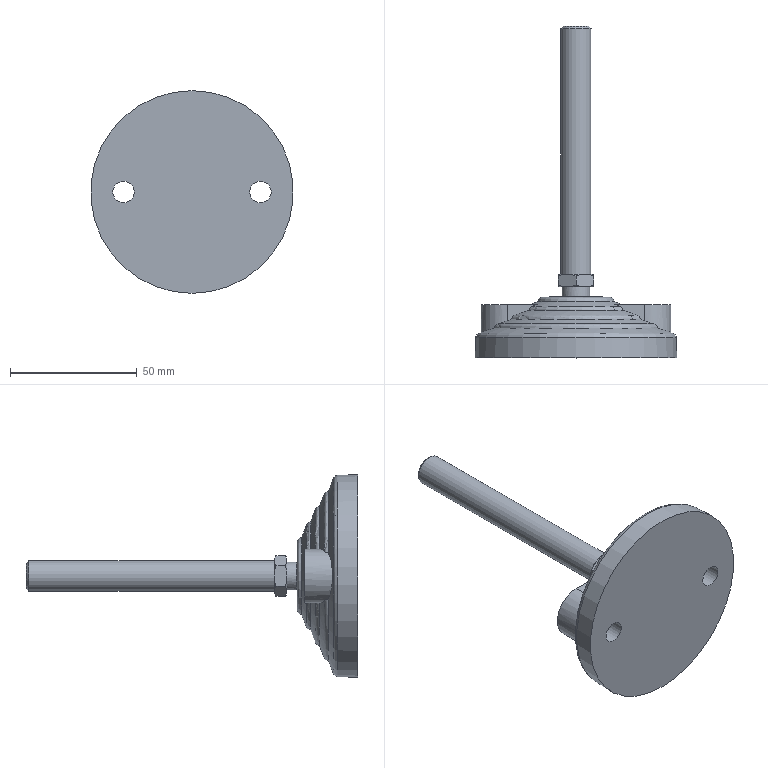Part | STEP file | Levelling elements for ground mounting LV.F-80-14-SST-M12x98(0) | 2 solids | 56 faces | box 80 x 131 x 80 mm | volume 93334 mm3 | cone 22 | plane 17 | torus 8 | cylinder 7 | sphere 2 | commonest cylinder face diameters 8.5 x2 21 x2 11 x1 12 x1 14 x1